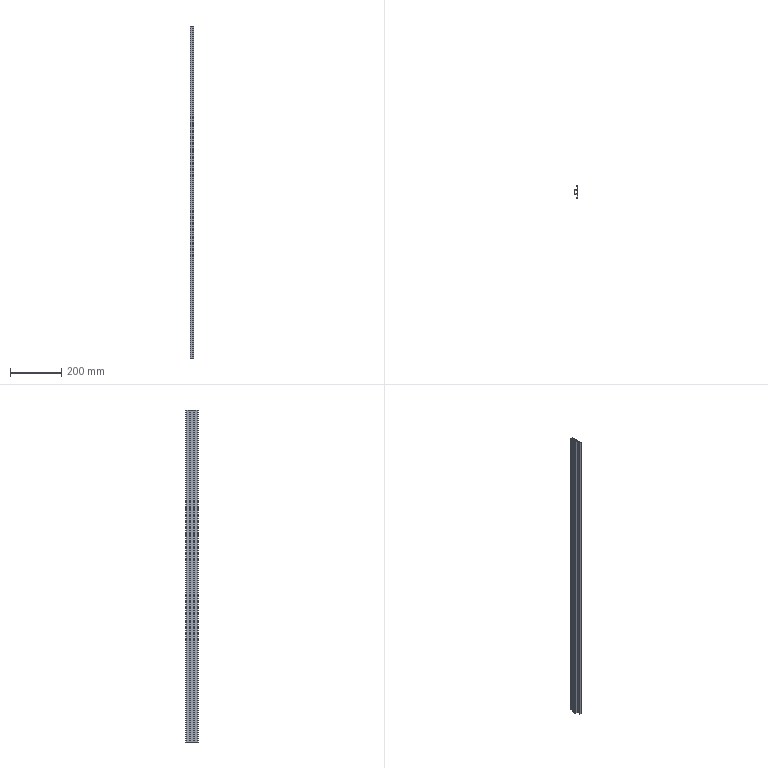Part | STEP file | Guide wheel mechanism revised.sldasm-Part-329 | 1 solid | 22 faces | box 14 x 50 x 1300 mm | volume 330720 mm3 | plane 22
STEP:
#1=CARTESIAN_POINT('',(0.,-7.,-650.));
#2=VERTEX_POINT('',#1);
#3=CARTESIAN_POINT('',(-8.,-7.,-650.));
#4=VERTEX_POINT('',#3);
#5=CARTESIAN_POINT('',(-8.,-7.,-650.));
#6=DIRECTION('',(-1.,0.,0.));
#7=VECTOR('',#6,1000.);
#8=LINE('',#5,#7);
#9=EDGE_CURVE('',#2,#4,#8,.T.);
#10=ORIENTED_EDGE('',*,*,#9,.T.);
#11=CARTESIAN_POINT('',(-8.,-7.,650.));
#12=VERTEX_POINT('',#11);
#13=CARTESIAN_POINT('',(-8.,-7.,650.));
#14=DIRECTION('',(0.,0.,-1.));
#15=VECTOR('',#14,1000.);
#16=LINE('',#13,#15);
#17=EDGE_CURVE('',#12,#4,#16,.T.);
#18=ORIENTED_EDGE('',*,*,#17,.F.);
#19=CARTESIAN_POINT('',(0.,-7.,650.));
#20=VERTEX_POINT('',#19);
#21=CARTESIAN_POINT('',(-8.,-7.,650.));
#22=DIRECTION('',(-1.,0.,0.));
#23=VECTOR('',#22,1000.);
#24=LINE('',#21,#23);
#25=EDGE_CURVE('',#20,#12,#24,.T.);
#26=ORIENTED_EDGE('',*,*,#25,.F.);
#27=CARTESIAN_POINT('',(0.,-7.,650.));
#28=DIRECTION('',(0.,0.,-1.));
#29=VECTOR('',#28,1000.);
#30=LINE('',#27,#29);
#31=EDGE_CURVE('',#20,#2,#30,.T.);
#32=ORIENTED_EDGE('',*,*,#31,.T.);
#33=EDGE_LOOP('',(#10,#18,#26,#32));
#34=FACE_OUTER_BOUND('',#33,.T.);
#35=CARTESIAN_POINT('',(-8.,-7.,650.));
#36=DIRECTION('',(0.,-1.,0.));
#37=DIRECTION('',(1.,0.,0.));
#38=AXIS2_PLACEMENT_3D('',#35,#36,#37);
#39=PLANE('',#38);
#40=ADVANCED_FACE('',(#34),#39,.F.);
#41=CARTESIAN_POINT('',(-8.,-4.6,-650.));
#42=VERTEX_POINT('',#41);
#43=CARTESIAN_POINT('',(-8.,-4.6,-650.));
#44=DIRECTION('',(0.,1.,0.));
#45=VECTOR('',#44,1000.);
#46=LINE('',#43,#45);
#47=EDGE_CURVE('',#4,#42,#46,.T.);
#48=ORIENTED_EDGE('',*,*,#47,.T.);
#49=CARTESIAN_POINT('',(-8.,-4.6,650.));
#50=VERTEX_POINT('',#49);
#51=CARTESIAN_POINT('',(-8.,-4.6,650.));
#52=DIRECTION('',(0.,0.,-1.));
#53=VECTOR('',#52,1000.);
#54=LINE('',#51,#53);
#55=EDGE_CURVE('',#50,#42,#54,.T.);
#56=ORIENTED_EDGE('',*,*,#55,.F.);
#57=CARTESIAN_POINT('',(-8.,-4.6,650.));
#58=DIRECTION('',(0.,1.,0.));
#59=VECTOR('',#58,1000.);
#60=LINE('',#57,#59);
#61=EDGE_CURVE('',#12,#50,#60,.T.);
#62=ORIENTED_EDGE('',*,*,#61,.F.);
#63=ORIENTED_EDGE('',*,*,#17,.T.);
#64=EDGE_LOOP('',(#48,#56,#62,#63));
#65=FACE_OUTER_BOUND('',#64,.T.);
#66=CARTESIAN_POINT('',(-8.,-4.6,650.));
#67=DIRECTION('',(-1.,0.,0.));
#68=DIRECTION('',(0.,0.,1.));
#69=AXIS2_PLACEMENT_3D('',#66,#67,#68);
#70=PLANE('',#69);
#71=ADVANCED_FACE('',(#65),#70,.F.);
#72=CARTESIAN_POINT('',(-11.,-4.6,-650.));
#73=VERTEX_POINT('',#72);
#74=CARTESIAN_POINT('',(-11.,-4.6,-650.));
#75=DIRECTION('',(-1.,0.,0.));
#76=VECTOR('',#75,1000.);
#77=LINE('',#74,#76);
#78=EDGE_CURVE('',#42,#73,#77,.T.);
#79=ORIENTED_EDGE('',*,*,#78,.T.);
#80=CARTESIAN_POINT('',(-11.,-4.6,650.));
#81=VERTEX_POINT('',#80);
#82=CARTESIAN_POINT('',(-11.,-4.6,650.));
#83=DIRECTION('',(0.,0.,-1.));
#84=VECTOR('',#83,1000.);
#85=LINE('',#82,#84);
#86=EDGE_CURVE('',#81,#73,#85,.T.);
#87=ORIENTED_EDGE('',*,*,#86,.F.);
#88=CARTESIAN_POINT('',(-11.,-4.6,650.));
#89=DIRECTION('',(-1.,0.,0.));
#90=VECTOR('',#89,1000.);
#91=LINE('',#88,#90);
#92=EDGE_CURVE('',#50,#81,#91,.T.);
#93=ORIENTED_EDGE('',*,*,#92,.F.);
#94=ORIENTED_EDGE('',*,*,#55,.T.);
#95=EDGE_LOOP('',(#79,#87,#93,#94));
#96=FACE_OUTER_BOUND('',#95,.T.);
#97=CARTESIAN_POINT('',(-11.,-4.6,650.));
#98=DIRECTION('',(0.,-1.,0.));
#99=DIRECTION('',(0.,0.,-1.));
#100=AXIS2_PLACEMENT_3D('',#97,#98,#99);
#101=PLANE('',#100);
#102=ADVANCED_FACE('',(#96),#101,.F.);
#103=CARTESIAN_POINT('',(-11.,-10.,-650.));
#104=VERTEX_POINT('',#103);
#105=CARTESIAN_POINT('',(-11.,-10.,-650.));
#106=DIRECTION('',(0.,-1.,0.));
#107=VECTOR('',#106,1000.);
#108=LINE('',#105,#107);
#109=EDGE_CURVE('',#73,#104,#108,.T.);
#110=ORIENTED_EDGE('',*,*,#109,.T.);
#111=CARTESIAN_POINT('',(-11.,-10.,650.));
#112=VERTEX_POINT('',#111);
#113=CARTESIAN_POINT('',(-11.,-10.,650.));
#114=DIRECTION('',(0.,0.,-1.));
#115=VECTOR('',#114,1000.);
#116=LINE('',#113,#115);
#117=EDGE_CURVE('',#112,#104,#116,.T.);
#118=ORIENTED_EDGE('',*,*,#117,.F.);
#119=CARTESIAN_POINT('',(-11.,-10.,650.));
#120=DIRECTION('',(0.,-1.,0.));
#121=VECTOR('',#120,1000.);
#122=LINE('',#119,#121);
#123=EDGE_CURVE('',#81,#112,#122,.T.);
#124=ORIENTED_EDGE('',*,*,#123,.F.);
#125=ORIENTED_EDGE('',*,*,#86,.T.);
#126=EDGE_LOOP('',(#110,#118,#124,#125));
#127=FACE_OUTER_BOUND('',#126,.T.);
#128=CARTESIAN_POINT('',(-11.,-10.,650.));
#129=DIRECTION('',(1.,0.,0.));
#130=DIRECTION('',(0.,1.,0.));
#131=AXIS2_PLACEMENT_3D('',#128,#129,#130);
#132=PLANE('',#131);
#133=ADVANCED_FACE('',(#127),#132,.F.);
#134=CARTESIAN_POINT('',(0.,-10.,-650.));
#135=VERTEX_POINT('',#134);
#136=CARTESIAN_POINT('',(0.,-10.,-650.));
#137=DIRECTION('',(1.,0.,0.));
#138=VECTOR('',#137,1000.);
#139=LINE('',#136,#138);
#140=EDGE_CURVE('',#104,#135,#139,.T.);
#141=ORIENTED_EDGE('',*,*,#140,.T.);
#142=CARTESIAN_POINT('',(0.,-10.,650.));
#143=VERTEX_POINT('',#142);
#144=CARTESIAN_POINT('',(0.,-10.,650.));
#145=DIRECTION('',(0.,0.,-1.));
#146=VECTOR('',#145,1000.);
#147=LINE('',#144,#146);
#148=EDGE_CURVE('',#143,#135,#147,.T.);
#149=ORIENTED_EDGE('',*,*,#148,.F.);
#150=CARTESIAN_POINT('',(0.,-10.,650.));
#151=DIRECTION('',(1.,0.,0.));
#152=VECTOR('',#151,1000.);
#153=LINE('',#150,#152);
#154=EDGE_CURVE('',#112,#143,#153,.T.);
#155=ORIENTED_EDGE('',*,*,#154,.F.);
#156=ORIENTED_EDGE('',*,*,#117,.T.);
#157=EDGE_LOOP('',(#141,#149,#155,#156));
#158=FACE_OUTER_BOUND('',#157,.T.);
#159=CARTESIAN_POINT('',(0.,-10.,650.));
#160=DIRECTION('',(0.,1.,0.));
#161=DIRECTION('',(-1.,0.,0.));
#162=AXIS2_PLACEMENT_3D('',#159,#160,#161);
#163=PLANE('',#162);
#164=ADVANCED_FACE('',(#158),#163,.F.);
#165=CARTESIAN_POINT('',(0.,-21.,-650.));
#166=VERTEX_POINT('',#165);
#167=CARTESIAN_POINT('',(0.,-21.,-650.));
#168=DIRECTION('',(0.,-1.,0.));
#169=VECTOR('',#168,1000.);
#170=LINE('',#167,#169);
#171=EDGE_CURVE('',#135,#166,#170,.T.);
#172=ORIENTED_EDGE('',*,*,#171,.T.);
#173=CARTESIAN_POINT('',(0.,-21.,650.));
#174=VERTEX_POINT('',#173);
#175=CARTESIAN_POINT('',(0.,-21.,650.));
#176=DIRECTION('',(0.,0.,-1.));
#177=VECTOR('',#176,1000.);
#178=LINE('',#175,#177);
#179=EDGE_CURVE('',#174,#166,#178,.T.);
#180=ORIENTED_EDGE('',*,*,#179,.F.);
#181=CARTESIAN_POINT('',(0.,-21.,650.));
#182=DIRECTION('',(0.,-1.,0.));
#183=VECTOR('',#182,1000.);
#184=LINE('',#181,#183);
#185=EDGE_CURVE('',#143,#174,#184,.T.);
#186=ORIENTED_EDGE('',*,*,#185,.F.);
#187=ORIENTED_EDGE('',*,*,#148,.T.);
#188=EDGE_LOOP('',(#172,#180,#186,#187));
#189=FACE_OUTER_BOUND('',#188,.T.);
#190=CARTESIAN_POINT('',(0.,-21.,650.));
#191=DIRECTION('',(1.,0.,0.));
#192=DIRECTION('',(0.,1.,0.));
#193=AXIS2_PLACEMENT_3D('',#190,#191,#192);
#194=PLANE('',#193);
#195=ADVANCED_FACE('',(#189),#194,.F.);
#196=CARTESIAN_POINT('',(-3.,-21.,-650.));
#197=VERTEX_POINT('',#196);
#198=CARTESIAN_POINT('',(-3.,-21.,-650.));
#199=DIRECTION('',(-1.,0.,0.));
#200=VECTOR('',#199,1000.);
#201=LINE('',#198,#200);
#202=EDGE_CURVE('',#166,#197,#201,.T.);
#203=ORIENTED_EDGE('',*,*,#202,.T.);
#204=CARTESIAN_POINT('',(-3.,-21.,650.));
#205=VERTEX_POINT('',#204);
#206=CARTESIAN_POINT('',(-3.,-21.,650.));
#207=DIRECTION('',(0.,0.,-1.));
#208=VECTOR('',#207,1000.);
#209=LINE('',#206,#208);
#210=EDGE_CURVE('',#205,#197,#209,.T.);
#211=ORIENTED_EDGE('',*,*,#210,.F.);
#212=CARTESIAN_POINT('',(-3.,-21.,650.));
#213=DIRECTION('',(-1.,0.,0.));
#214=VECTOR('',#213,1000.);
#215=LINE('',#212,#214);
#216=EDGE_CURVE('',#174,#205,#215,.T.);
#217=ORIENTED_EDGE('',*,*,#216,.F.);
#218=ORIENTED_EDGE('',*,*,#179,.T.);
#219=EDGE_LOOP('',(#203,#211,#217,#218));
#220=FACE_OUTER_BOUND('',#219,.T.);
#221=CARTESIAN_POINT('',(-3.,-21.,650.));
#222=DIRECTION('',(0.,-1.,0.));
#223=DIRECTION('',(1.,0.,0.));
#224=AXIS2_PLACEMENT_3D('',#221,#222,#223);
#225=PLANE('',#224);
#226=ADVANCED_FACE('',(#220),#225,.F.);
#227=CARTESIAN_POINT('',(-3.,-25.,-650.));
#228=VERTEX_POINT('',#227);
#229=CARTESIAN_POINT('',(-3.,-25.,-650.));
#230=DIRECTION('',(0.,-1.,0.));
#231=VECTOR('',#230,1000.);
#232=LINE('',#229,#231);
#233=EDGE_CURVE('',#197,#228,#232,.T.);
#234=ORIENTED_EDGE('',*,*,#233,.T.);
#235=CARTESIAN_POINT('',(-3.,-25.,650.));
#236=VERTEX_POINT('',#235);
#237=CARTESIAN_POINT('',(-3.,-25.,650.));
#238=DIRECTION('',(0.,0.,-1.));
#239=VECTOR('',#238,1000.);
#240=LINE('',#237,#239);
#241=EDGE_CURVE('',#236,#228,#240,.T.);
#242=ORIENTED_EDGE('',*,*,#241,.F.);
#243=CARTESIAN_POINT('',(-3.,-25.,650.));
#244=DIRECTION('',(0.,-1.,0.));
#245=VECTOR('',#244,1000.);
#246=LINE('',#243,#245);
#247=EDGE_CURVE('',#205,#236,#246,.T.);
#248=ORIENTED_EDGE('',*,*,#247,.F.);
#249=ORIENTED_EDGE('',*,*,#210,.T.);
#250=EDGE_LOOP('',(#234,#242,#248,#249));
#251=FACE_OUTER_BOUND('',#250,.T.);
#252=CARTESIAN_POINT('',(-3.,-25.,650.));
#253=DIRECTION('',(1.,0.,0.));
#254=DIRECTION('',(0.,0.,-1.));
#255=AXIS2_PLACEMENT_3D('',#252,#253,#254);
#256=PLANE('',#255);
#257=ADVANCED_FACE('',(#251),#256,.F.);
#258=CARTESIAN_POINT('',(3.,-25.,-650.));
#259=VERTEX_POINT('',#258);
#260=CARTESIAN_POINT('',(3.,-25.,-650.));
#261=DIRECTION('',(1.,0.,0.));
#262=VECTOR('',#261,1000.);
#263=LINE('',#260,#262);
#264=EDGE_CURVE('',#228,#259,#263,.T.);
#265=ORIENTED_EDGE('',*,*,#264,.T.);
#266=CARTESIAN_POINT('',(3.,-25.,650.));
#267=VERTEX_POINT('',#266);
#268=CARTESIAN_POINT('',(3.,-25.,650.));
#269=DIRECTION('',(0.,0.,-1.));
#270=VECTOR('',#269,1000.);
#271=LINE('',#268,#270);
#272=EDGE_CURVE('',#267,#259,#271,.T.);
#273=ORIENTED_EDGE('',*,*,#272,.F.);
#274=CARTESIAN_POINT('',(3.,-25.,650.));
#275=DIRECTION('',(1.,0.,0.));
#276=VECTOR('',#275,1000.);
#277=LINE('',#274,#276);
#278=EDGE_CURVE('',#236,#267,#277,.T.);
#279=ORIENTED_EDGE('',*,*,#278,.F.);
#280=ORIENTED_EDGE('',*,*,#241,.T.);
#281=EDGE_LOOP('',(#265,#273,#279,#280));
#282=FACE_OUTER_BOUND('',#281,.T.);
#283=CARTESIAN_POINT('',(3.,-25.,650.));
#284=DIRECTION('',(0.,1.,0.));
#285=DIRECTION('',(0.,0.,1.));
#286=AXIS2_PLACEMENT_3D('',#283,#284,#285);
#287=PLANE('',#286);
#288=ADVANCED_FACE('',(#282),#287,.F.);
#289=CARTESIAN_POINT('',(3.,25.,-650.));
#290=VERTEX_POINT('',#289);
#291=CARTESIAN_POINT('',(3.,-25.,-650.));
#292=DIRECTION('',(0.,1.,0.));
#293=VECTOR('',#292,1000.);
#294=LINE('',#291,#293);
#295=EDGE_CURVE('',#259,#290,#294,.T.);
#296=ORIENTED_EDGE('',*,*,#295,.T.);
#297=CARTESIAN_POINT('',(3.,25.,650.));
#298=VERTEX_POINT('',#297);
#299=CARTESIAN_POINT('',(3.,25.,650.));
#300=DIRECTION('',(0.,0.,-1.));
#301=VECTOR('',#300,1000.);
#302=LINE('',#299,#301);
#303=EDGE_CURVE('',#298,#290,#302,.T.);
#304=ORIENTED_EDGE('',*,*,#303,.F.);
#305=CARTESIAN_POINT('',(3.,-25.,650.));
#306=DIRECTION('',(0.,1.,0.));
#307=VECTOR('',#306,1000.);
#308=LINE('',#305,#307);
#309=EDGE_CURVE('',#267,#298,#308,.T.);
#310=ORIENTED_EDGE('',*,*,#309,.F.);
#311=ORIENTED_EDGE('',*,*,#272,.T.);
#312=EDGE_LOOP('',(#296,#304,#310,#311));
#313=FACE_OUTER_BOUND('',#312,.T.);
#314=CARTESIAN_POINT('',(3.,-25.,650.));
#315=DIRECTION('',(-1.,0.,0.));
#316=DIRECTION('',(0.,0.,1.));
#317=AXIS2_PLACEMENT_3D('',#314,#315,#316);
#318=PLANE('',#317);
#319=ADVANCED_FACE('',(#313),#318,.F.);
#320=CARTESIAN_POINT('',(-3.,25.,-650.));
#321=VERTEX_POINT('',#320);
#322=CARTESIAN_POINT('',(3.,25.,-650.));
#323=DIRECTION('',(-1.,0.,0.));
#324=VECTOR('',#323,1000.);
#325=LINE('',#322,#324);
#326=EDGE_CURVE('',#290,#321,#325,.T.);
#327=ORIENTED_EDGE('',*,*,#326,.T.);
#328=CARTESIAN_POINT('',(-3.,25.,650.));
#329=VERTEX_POINT('',#328);
#330=CARTESIAN_POINT('',(-3.,25.,650.));
#331=DIRECTION('',(0.,0.,-1.));
#332=VECTOR('',#331,1000.);
#333=LINE('',#330,#332);
#334=EDGE_CURVE('',#329,#321,#333,.T.);
#335=ORIENTED_EDGE('',*,*,#334,.F.);
#336=CARTESIAN_POINT('',(3.,25.,650.));
#337=DIRECTION('',(-1.,0.,0.));
#338=VECTOR('',#337,1000.);
#339=LINE('',#336,#338);
#340=EDGE_CURVE('',#298,#329,#339,.T.);
#341=ORIENTED_EDGE('',*,*,#340,.F.);
#342=ORIENTED_EDGE('',*,*,#303,.T.);
#343=EDGE_LOOP('',(#327,#335,#341,#342));
#344=FACE_OUTER_BOUND('',#343,.T.);
#345=CARTESIAN_POINT('',(3.,25.,650.));
#346=DIRECTION('',(0.,-1.,0.));
#347=DIRECTION('',(0.,0.,-1.));
#348=AXIS2_PLACEMENT_3D('',#345,#346,#347);
#349=PLANE('',#348);
#350=ADVANCED_FACE('',(#344),#349,.F.);
#351=CARTESIAN_POINT('',(-3.,21.,-650.));
#352=VERTEX_POINT('',#351);
#353=CARTESIAN_POINT('',(-3.,25.,-650.));
#354=DIRECTION('',(0.,-1.,0.));
#355=VECTOR('',#354,1000.);
#356=LINE('',#353,#355);
#357=EDGE_CURVE('',#321,#352,#356,.T.);
#358=ORIENTED_EDGE('',*,*,#357,.T.);
#359=CARTESIAN_POINT('',(-3.,21.,650.));
#360=VERTEX_POINT('',#359);
#361=CARTESIAN_POINT('',(-3.,21.,650.));
#362=DIRECTION('',(0.,0.,-1.));
#363=VECTOR('',#362,1000.);
#364=LINE('',#361,#363);
#365=EDGE_CURVE('',#360,#352,#364,.T.);
#366=ORIENTED_EDGE('',*,*,#365,.F.);
#367=CARTESIAN_POINT('',(-3.,25.,650.));
#368=DIRECTION('',(0.,-1.,0.));
#369=VECTOR('',#368,1000.);
#370=LINE('',#367,#369);
#371=EDGE_CURVE('',#329,#360,#370,.T.);
#372=ORIENTED_EDGE('',*,*,#371,.F.);
#373=ORIENTED_EDGE('',*,*,#334,.T.);
#374=EDGE_LOOP('',(#358,#366,#372,#373));
#375=FACE_OUTER_BOUND('',#374,.T.);
#376=CARTESIAN_POINT('',(-3.,25.,650.));
#377=DIRECTION('',(1.,0.,0.));
#378=DIRECTION('',(0.,0.,-1.));
#379=AXIS2_PLACEMENT_3D('',#376,#377,#378);
#380=PLANE('',#379);
#381=ADVANCED_FACE('',(#375),#380,.F.);
#382=CARTESIAN_POINT('',(0.,21.,-650.));
#383=VERTEX_POINT('',#382);
#384=CARTESIAN_POINT('',(-3.,21.,-650.));
#385=DIRECTION('',(1.,0.,0.));
#386=VECTOR('',#385,1000.);
#387=LINE('',#384,#386);
#388=EDGE_CURVE('',#352,#383,#387,.T.);
#389=ORIENTED_EDGE('',*,*,#388,.T.);
#390=CARTESIAN_POINT('',(0.,21.,650.));
#391=VERTEX_POINT('',#390);
#392=CARTESIAN_POINT('',(0.,21.,650.));
#393=DIRECTION('',(0.,0.,-1.));
#394=VECTOR('',#393,1000.);
#395=LINE('',#392,#394);
#396=EDGE_CURVE('',#391,#383,#395,.T.);
#397=ORIENTED_EDGE('',*,*,#396,.F.);
#398=CARTESIAN_POINT('',(-3.,21.,650.));
#399=DIRECTION('',(1.,0.,0.));
#400=VECTOR('',#399,1000.);
#401=LINE('',#398,#400);
#402=EDGE_CURVE('',#360,#391,#401,.T.);
#403=ORIENTED_EDGE('',*,*,#402,.F.);
#404=ORIENTED_EDGE('',*,*,#365,.T.);
#405=EDGE_LOOP('',(#389,#397,#403,#404));
#406=FACE_OUTER_BOUND('',#405,.T.);
#407=CARTESIAN_POINT('',(-3.,21.,650.));
#408=DIRECTION('',(0.,1.,0.));
#409=DIRECTION('',(-1.,0.,0.));
#410=AXIS2_PLACEMENT_3D('',#407,#408,#409);
#411=PLANE('',#410);
#412=ADVANCED_FACE('',(#406),#411,.F.);
#413=CARTESIAN_POINT('',(0.,10.,-650.));
#414=VERTEX_POINT('',#413);
#415=CARTESIAN_POINT('',(0.,21.,-650.));
#416=DIRECTION('',(0.,-1.,0.));
#417=VECTOR('',#416,1000.);
#418=LINE('',#415,#417);
#419=EDGE_CURVE('',#383,#414,#418,.T.);
#420=ORIENTED_EDGE('',*,*,#419,.T.);
#421=CARTESIAN_POINT('',(0.,10.,650.));
#422=VERTEX_POINT('',#421);
#423=CARTESIAN_POINT('',(0.,10.,650.));
#424=DIRECTION('',(0.,0.,-1.));
#425=VECTOR('',#424,1000.);
#426=LINE('',#423,#425);
#427=EDGE_CURVE('',#422,#414,#426,.T.);
#428=ORIENTED_EDGE('',*,*,#427,.F.);
#429=CARTESIAN_POINT('',(0.,21.,650.));
#430=DIRECTION('',(0.,-1.,0.));
#431=VECTOR('',#430,1000.);
#432=LINE('',#429,#431);
#433=EDGE_CURVE('',#391,#422,#432,.T.);
#434=ORIENTED_EDGE('',*,*,#433,.F.);
#435=ORIENTED_EDGE('',*,*,#396,.T.);
#436=EDGE_LOOP('',(#420,#428,#434,#435));
#437=FACE_OUTER_BOUND('',#436,.T.);
#438=CARTESIAN_POINT('',(0.,21.,650.));
#439=DIRECTION('',(1.,0.,0.));
#440=DIRECTION('',(0.,1.,0.));
#441=AXIS2_PLACEMENT_3D('',#438,#439,#440);
#442=PLANE('',#441);
#443=ADVANCED_FACE('',(#437),#442,.F.);
#444=CARTESIAN_POINT('',(-11.,10.,-650.));
#445=VERTEX_POINT('',#444);
#446=CARTESIAN_POINT('',(0.,10.,-650.));
#447=DIRECTION('',(-1.,0.,0.));
#448=VECTOR('',#447,1000.);
#449=LINE('',#446,#448);
#450=EDGE_CURVE('',#414,#445,#449,.T.);
#451=ORIENTED_EDGE('',*,*,#450,.T.);
#452=CARTESIAN_POINT('',(-11.,10.,650.));
#453=VERTEX_POINT('',#452);
#454=CARTESIAN_POINT('',(-11.,10.,650.));
#455=DIRECTION('',(0.,0.,-1.));
#456=VECTOR('',#455,1000.);
#457=LINE('',#454,#456);
#458=EDGE_CURVE('',#453,#445,#457,.T.);
#459=ORIENTED_EDGE('',*,*,#458,.F.);
#460=CARTESIAN_POINT('',(0.,10.,650.));
#461=DIRECTION('',(-1.,0.,0.));
#462=VECTOR('',#461,1000.);
#463=LINE('',#460,#462);
#464=EDGE_CURVE('',#422,#453,#463,.T.);
#465=ORIENTED_EDGE('',*,*,#464,.F.);
#466=ORIENTED_EDGE('',*,*,#427,.T.);
#467=EDGE_LOOP('',(#451,#459,#465,#466));
#468=FACE_OUTER_BOUND('',#467,.T.);
#469=CARTESIAN_POINT('',(0.,10.,650.));
#470=DIRECTION('',(0.,-1.,0.));
#471=DIRECTION('',(1.,0.,0.));
#472=AXIS2_PLACEMENT_3D('',#469,#470,#471);
#473=PLANE('',#472);
#474=ADVANCED_FACE('',(#468),#473,.F.);
#475=CARTESIAN_POINT('',(-11.,4.6,-650.));
#476=VERTEX_POINT('',#475);
#477=CARTESIAN_POINT('',(-11.,10.,-650.));
#478=DIRECTION('',(0.,-1.,0.));
#479=VECTOR('',#478,1000.);
#480=LINE('',#477,#479);
#481=EDGE_CURVE('',#445,#476,#480,.T.);
#482=ORIENTED_EDGE('',*,*,#481,.T.);
#483=CARTESIAN_POINT('',(-11.,4.6,650.));
#484=VERTEX_POINT('',#483);
#485=CARTESIAN_POINT('',(-11.,4.6,650.));
#486=DIRECTION('',(0.,0.,-1.));
#487=VECTOR('',#486,1000.);
#488=LINE('',#485,#487);
#489=EDGE_CURVE('',#484,#476,#488,.T.);
#490=ORIENTED_EDGE('',*,*,#489,.F.);
#491=CARTESIAN_POINT('',(-11.,10.,650.));
#492=DIRECTION('',(0.,-1.,0.));
#493=VECTOR('',#492,1000.);
#494=LINE('',#491,#493);
#495=EDGE_CURVE('',#453,#484,#494,.T.);
#496=ORIENTED_EDGE('',*,*,#495,.F.);
#497=ORIENTED_EDGE('',*,*,#458,.T.);
#498=EDGE_LOOP('',(#482,#490,#496,#497));
#499=FACE_OUTER_BOUND('',#498,.T.);
#500=CARTESIAN_POINT('',(-11.,10.,650.));
#501=DIRECTION('',(1.,0.,0.));
#502=DIRECTION('',(0.,1.,0.));
#503=AXIS2_PLACEMENT_3D('',#500,#501,#502);
#504=PLANE('',#503);
#505=ADVANCED_FACE('',(#499),#504,.F.);
#506=CARTESIAN_POINT('',(-8.,4.6,-650.));
#507=VERTEX_POINT('',#506);
#508=CARTESIAN_POINT('',(-11.,4.6,-650.));
#509=DIRECTION('',(1.,0.,0.));
#510=VECTOR('',#509,1000.);
#511=LINE('',#508,#510);
#512=EDGE_CURVE('',#476,#507,#511,.T.);
#513=ORIENTED_EDGE('',*,*,#512,.T.);
#514=CARTESIAN_POINT('',(-8.,4.6,650.));
#515=VERTEX_POINT('',#514);
#516=CARTESIAN_POINT('',(-8.,4.6,650.));
#517=DIRECTION('',(0.,0.,-1.));
#518=VECTOR('',#517,1000.);
#519=LINE('',#516,#518);
#520=EDGE_CURVE('',#515,#507,#519,.T.);
#521=ORIENTED_EDGE('',*,*,#520,.F.);
#522=CARTESIAN_POINT('',(-11.,4.6,650.));
#523=DIRECTION('',(1.,0.,0.));
#524=VECTOR('',#523,1000.);
#525=LINE('',#522,#524);
#526=EDGE_CURVE('',#484,#515,#525,.T.);
#527=ORIENTED_EDGE('',*,*,#526,.F.);
#528=ORIENTED_EDGE('',*,*,#489,.T.);
#529=EDGE_LOOP('',(#513,#521,#527,#528));
#530=FACE_OUTER_BOUND('',#529,.T.);
#531=CARTESIAN_POINT('',(-11.,4.6,650.));
#532=DIRECTION('',(0.,1.,0.));
#533=DIRECTION('',(0.,0.,1.));
#534=AXIS2_PLACEMENT_3D('',#531,#532,#533);
#535=PLANE('',#534);
#536=ADVANCED_FACE('',(#530),#535,.F.);
#537=CARTESIAN_POINT('',(-8.,7.,-650.));
#538=VERTEX_POINT('',#537);
#539=CARTESIAN_POINT('',(-8.,4.6,-650.));
#540=DIRECTION('',(0.,1.,0.));
#541=VECTOR('',#540,1000.);
#542=LINE('',#539,#541);
#543=EDGE_CURVE('',#507,#538,#542,.T.);
#544=ORIENTED_EDGE('',*,*,#543,.T.);
#545=CARTESIAN_POINT('',(-8.,7.,650.));
#546=VERTEX_POINT('',#545);
#547=CARTESIAN_POINT('',(-8.,7.,650.));
#548=DIRECTION('',(0.,0.,-1.));
#549=VECTOR('',#548,1000.);
#550=LINE('',#547,#549);
#551=EDGE_CURVE('',#546,#538,#550,.T.);
#552=ORIENTED_EDGE('',*,*,#551,.F.);
#553=CARTESIAN_POINT('',(-8.,4.6,650.));
#554=DIRECTION('',(0.,1.,0.));
#555=VECTOR('',#554,1000.);
#556=LINE('',#553,#555);
#557=EDGE_CURVE('',#515,#546,#556,.T.);
#558=ORIENTED_EDGE('',*,*,#557,.F.);
#559=ORIENTED_EDGE('',*,*,#520,.T.);
#560=EDGE_LOOP('',(#544,#552,#558,#559));
#561=FACE_OUTER_BOUND('',#560,.T.);
#562=CARTESIAN_POINT('',(-8.,4.6,650.));
#563=DIRECTION('',(-1.,0.,0.));
#564=DIRECTION('',(0.,0.,1.));
#565=AXIS2_PLACEMENT_3D('',#562,#563,#564);
#566=PLANE('',#565);
#567=ADVANCED_FACE('',(#561),#566,.F.);
#568=CARTESIAN_POINT('',(0.,7.,-650.));
#569=VERTEX_POINT('',#568);
#570=CARTESIAN_POINT('',(-8.,7.,-650.));
#571=DIRECTION('',(1.,0.,0.));
#572=VECTOR('',#571,1000.);
#573=LINE('',#570,#572);
#574=EDGE_CURVE('',#538,#569,#573,.T.);
#575=ORIENTED_EDGE('',*,*,#574,.T.);
#576=CARTESIAN_POINT('',(0.,7.,650.));
#577=VERTEX_POINT('',#576);
#578=CARTESIAN_POINT('',(0.,7.,650.));
#579=DIRECTION('',(0.,0.,-1.));
#580=VECTOR('',#579,1000.);
#581=LINE('',#578,#580);
#582=EDGE_CURVE('',#577,#569,#581,.T.);
#583=ORIENTED_EDGE('',*,*,#582,.F.);
#584=CARTESIAN_POINT('',(-8.,7.,650.));
#585=DIRECTION('',(1.,0.,0.));
#586=VECTOR('',#585,1000.);
#587=LINE('',#584,#586);
#588=EDGE_CURVE('',#546,#577,#587,.T.);
#589=ORIENTED_EDGE('',*,*,#588,.F.);
#590=ORIENTED_EDGE('',*,*,#551,.T.);
#591=EDGE_LOOP('',(#575,#583,#589,#590));
#592=FACE_OUTER_BOUND('',#591,.T.);
#593=CARTESIAN_POINT('',(-8.,7.,650.));
#594=DIRECTION('',(0.,1.,0.));
#595=DIRECTION('',(-1.,0.,0.));
#596=AXIS2_PLACEMENT_3D('',#593,#594,#595);
#597=PLANE('',#596);
#598=ADVANCED_FACE('',(#592),#597,.F.);
#599=CARTESIAN_POINT('',(0.,7.,-650.));
#600=DIRECTION('',(0.,-1.,0.));
#601=VECTOR('',#600,1000.);
#602=LINE('',#599,#601);
#603=EDGE_CURVE('',#569,#2,#602,.T.);
#604=ORIENTED_EDGE('',*,*,#603,.T.);
#605=ORIENTED_EDGE('',*,*,#31,.F.);
#606=CARTESIAN_POINT('',(0.,7.,650.));
#607=DIRECTION('',(0.,-1.,0.));
#608=VECTOR('',#607,1000.);
#609=LINE('',#606,#608);
#610=EDGE_CURVE('',#577,#20,#609,.T.);
#611=ORIENTED_EDGE('',*,*,#610,.F.);
#612=ORIENTED_EDGE('',*,*,#582,.T.);
#613=EDGE_LOOP('',(#604,#605,#611,#612));
#614=FACE_OUTER_BOUND('',#613,.T.);
#615=CARTESIAN_POINT('',(0.,7.,650.));
#616=DIRECTION('',(1.,0.,0.));
#617=DIRECTION('',(0.,0.,-1.));
#618=AXIS2_PLACEMENT_3D('',#615,#616,#617);
#619=PLANE('',#618);
#620=ADVANCED_FACE('',(#614),#619,.F.);
#621=ORIENTED_EDGE('',*,*,#25,.T.);
#622=ORIENTED_EDGE('',*,*,#61,.T.);
#623=ORIENTED_EDGE('',*,*,#92,.T.);
#624=ORIENTED_EDGE('',*,*,#123,.T.);
#625=ORIENTED_EDGE('',*,*,#154,.T.);
#626=ORIENTED_EDGE('',*,*,#185,.T.);
#627=ORIENTED_EDGE('',*,*,#216,.T.);
#628=ORIENTED_EDGE('',*,*,#247,.T.);
#629=ORIENTED_EDGE('',*,*,#278,.T.);
#630=ORIENTED_EDGE('',*,*,#309,.T.);
#631=ORIENTED_EDGE('',*,*,#340,.T.);
#632=ORIENTED_EDGE('',*,*,#371,.T.);
#633=ORIENTED_EDGE('',*,*,#402,.T.);
#634=ORIENTED_EDGE('',*,*,#433,.T.);
#635=ORIENTED_EDGE('',*,*,#464,.T.);
#636=ORIENTED_EDGE('',*,*,#495,.T.);
#637=ORIENTED_EDGE('',*,*,#526,.T.);
#638=ORIENTED_EDGE('',*,*,#557,.T.);
#639=ORIENTED_EDGE('',*,*,#588,.T.);
#640=ORIENTED_EDGE('',*,*,#610,.T.);
#641=EDGE_LOOP('',(#621,#622,#623,#624,#625,#626,#627,#628,#629,#630,#631,#632,#633,#634,#635,#636,#637,#638,#639,#640));
#642=FACE_OUTER_BOUND('',#641,.T.);
#643=CARTESIAN_POINT('',(0.,0.,650.));
#644=DIRECTION('',(0.,0.,-1.));
#645=DIRECTION('',(-1.,0.,0.));
#646=AXIS2_PLACEMENT_3D('',#643,#644,#645);
#647=PLANE('',#646);
#648=ADVANCED_FACE('',(#642),#647,.F.);
#649=ORIENTED_EDGE('',*,*,#9,.F.);
#650=ORIENTED_EDGE('',*,*,#603,.F.);
#651=ORIENTED_EDGE('',*,*,#574,.F.);
#652=ORIENTED_EDGE('',*,*,#543,.F.);
#653=ORIENTED_EDGE('',*,*,#512,.F.);
#654=ORIENTED_EDGE('',*,*,#481,.F.);
#655=ORIENTED_EDGE('',*,*,#450,.F.);
#656=ORIENTED_EDGE('',*,*,#419,.F.);
#657=ORIENTED_EDGE('',*,*,#388,.F.);
#658=ORIENTED_EDGE('',*,*,#357,.F.);
#659=ORIENTED_EDGE('',*,*,#326,.F.);
#660=ORIENTED_EDGE('',*,*,#295,.F.);
#661=ORIENTED_EDGE('',*,*,#264,.F.);
#662=ORIENTED_EDGE('',*,*,#233,.F.);
#663=ORIENTED_EDGE('',*,*,#202,.F.);
#664=ORIENTED_EDGE('',*,*,#171,.F.);
#665=ORIENTED_EDGE('',*,*,#140,.F.);
#666=ORIENTED_EDGE('',*,*,#109,.F.);
#667=ORIENTED_EDGE('',*,*,#78,.F.);
#668=ORIENTED_EDGE('',*,*,#47,.F.);
#669=EDGE_LOOP('',(#649,#650,#651,#652,#653,#654,#655,#656,#657,#658,#659,#660,#661,#662,#663,#664,#665,#666,#667,#668));
#670=FACE_OUTER_BOUND('',#669,.T.);
#671=CARTESIAN_POINT('',(0.,0.,-650.));
#672=DIRECTION('',(0.,0.,-1.));
#673=DIRECTION('',(-1.,0.,0.));
#674=AXIS2_PLACEMENT_3D('',#671,#672,#673);
#675=PLANE('',#674);
#676=ADVANCED_FACE('',(#670),#675,.T.);
#677=CLOSED_SHELL('',(#40,#71,#102,#133,#164,#195,#226,#257,#288,#319,#350,#381,#412,#443,#474,#505,#536,#567,#598,#620,#648,#676));
#678=MANIFOLD_SOLID_BREP('',#677);
#679=CARTESIAN_POINT('',(0.,0.,0.));
#680=DIRECTION('',(0.,0.,1.));
#681=DIRECTION('',(1.,0.,0.));
#682=AXIS2_PLACEMENT_3D('',#679,#680,#681);
#683=(LENGTH_UNIT()NAMED_UNIT(*)SI_UNIT(.MILLI.,.METRE.));
#684=UNCERTAINTY_MEASURE_WITH_UNIT(LENGTH_MEASURE(0.00001),#683,'','');
#685=(NAMED_UNIT(*)PLANE_ANGLE_UNIT()SI_UNIT($,.RADIAN.));
#686=(NAMED_UNIT(*)SI_UNIT($,.STERADIAN.)SOLID_ANGLE_UNIT());
#687=(GEOMETRIC_REPRESENTATION_CONTEXT(3)GLOBAL_UNCERTAINTY_ASSIGNED_CONTEXT((#684))GLOBAL_UNIT_ASSIGNED_CONTEXT((#683,#685,#686))REPRESENTATION_CONTEXT('',''));
#688=ADVANCED_BREP_SHAPE_REPRESENTATION('',(#678,#682),#687);